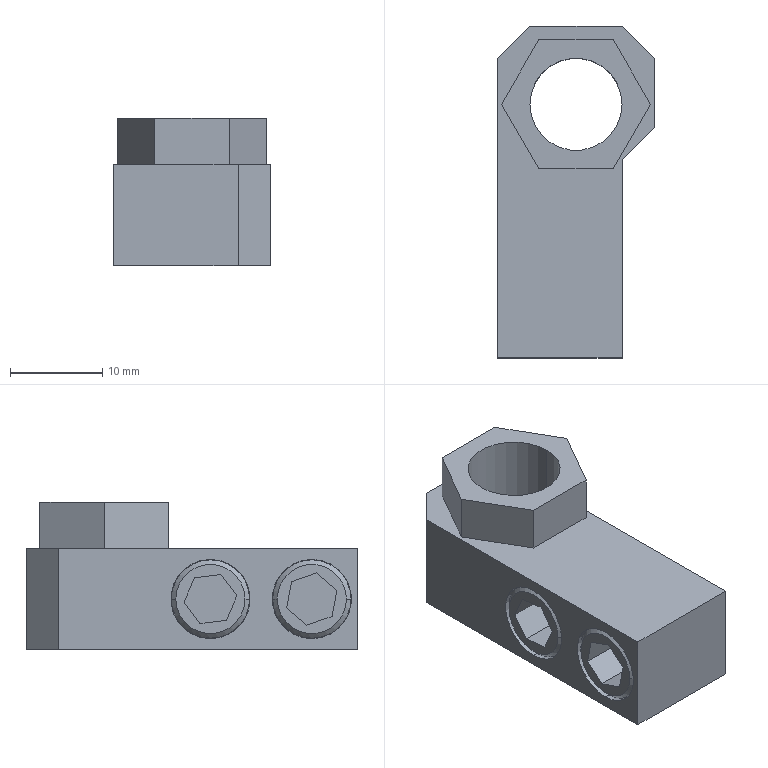Part | NX | 1 solid | 49 faces | box 17 x 36 x 16 mm | volume 4849 mm3 | plane 35 | cylinder 10 | cone 4 | commonest cylinder face diameters 8.5 x4 8.6 x4 10 x2
STEP:
#1=CARTESIAN_POINT('',(0.,27.5,10.5));
#2=VERTEX_POINT('',#1);
#3=CARTESIAN_POINT('',(-10.,27.5,10.5));
#4=VERTEX_POINT('',#3);
#5=CARTESIAN_POINT('',(-5.,27.5,10.5));
#6=DIRECTION('',(0.,0.,1.));
#7=DIRECTION('',(1.,0.,0.));
#8=AXIS2_PLACEMENT_3D('',#5,#6,#7);
#9=CIRCLE('',#8,5.);
#10=EDGE_CURVE('',#2,#4,#9,.T.);
#11=ORIENTED_EDGE('',*,*,#10,.T.);
#12=CARTESIAN_POINT('',(-10.,27.5,-5.5));
#13=VERTEX_POINT('',#12);
#14=CARTESIAN_POINT('',(-10.,27.5,-5.5));
#15=DIRECTION('',(0.,0.,1.));
#16=VECTOR('',#15,1000.);
#17=LINE('',#14,#16);
#18=EDGE_CURVE('',#4,#13,#17,.F.);
#19=ORIENTED_EDGE('',*,*,#18,.T.);
#20=CARTESIAN_POINT('',(0.,27.5,-5.5));
#21=VERTEX_POINT('',#20);
#22=CARTESIAN_POINT('',(-5.,27.5,-5.5));
#23=DIRECTION('',(0.,0.,1.));
#24=DIRECTION('',(1.,0.,0.));
#25=AXIS2_PLACEMENT_3D('',#22,#23,#24);
#26=CIRCLE('',#25,5.);
#27=EDGE_CURVE('',#21,#13,#26,.T.);
#28=ORIENTED_EDGE('',*,*,#27,.F.);
#29=CARTESIAN_POINT('',(0.,27.5,-5.5));
#30=DIRECTION('',(0.,0.,1.));
#31=VECTOR('',#30,1000.);
#32=LINE('',#29,#31);
#33=EDGE_CURVE('',#2,#21,#32,.F.);
#34=ORIENTED_EDGE('',*,*,#33,.F.);
#35=EDGE_LOOP('',(#11,#19,#28,#34));
#36=FACE_BOUND('',#35,.T.);
#37=CARTESIAN_POINT('',(-5.,27.5,-5.5));
#38=DIRECTION('',(0.,0.,1.));
#39=DIRECTION('',(1.,0.,0.));
#40=AXIS2_PLACEMENT_3D('',#37,#38,#39);
#41=CYLINDRICAL_SURFACE('',#40,5.);
#42=ADVANCED_FACE('',(#36),#41,.F.);
#43=CARTESIAN_POINT('',(-13.5,8.75,0.));
#44=VERTEX_POINT('',#43);
#45=CARTESIAN_POINT('',(-13.5,1.25,0.));
#46=VERTEX_POINT('',#45);
#47=CARTESIAN_POINT('',(-13.5,5.,0.));
#48=DIRECTION('',(-1.,0.,0.));
#49=DIRECTION('',(0.,0.,1.));
#50=AXIS2_PLACEMENT_3D('',#47,#48,#49);
#51=CIRCLE('',#50,3.75);
#52=EDGE_CURVE('',#44,#46,#51,.T.);
#53=ORIENTED_EDGE('',*,*,#52,.F.);
#54=CARTESIAN_POINT('',(-13.,9.25,0.));
#55=VERTEX_POINT('',#54);
#56=CARTESIAN_POINT('',(-13.5,8.75,0.));
#57=DIRECTION('',(0.7071,0.7071,0.));
#58=VECTOR('',#57,1000.);
#59=LINE('',#56,#58);
#60=EDGE_CURVE('',#44,#55,#59,.T.);
#61=ORIENTED_EDGE('',*,*,#60,.T.);
#62=CARTESIAN_POINT('',(-13.,5.,-4.25));
#63=VERTEX_POINT('',#62);
#64=CARTESIAN_POINT('',(-13.,5.,0.));
#65=DIRECTION('',(1.,0.,0.));
#66=DIRECTION('',(0.,0.,1.));
#67=AXIS2_PLACEMENT_3D('',#64,#65,#66);
#68=CIRCLE('',#67,4.25);
#69=EDGE_CURVE('',#63,#55,#68,.T.);
#70=ORIENTED_EDGE('',*,*,#69,.F.);
#71=CARTESIAN_POINT('',(-13.,0.75,0.));
#72=VERTEX_POINT('',#71);
#73=CARTESIAN_POINT('',(-13.,5.,0.));
#74=DIRECTION('',(1.,0.,0.));
#75=DIRECTION('',(0.,0.,1.));
#76=AXIS2_PLACEMENT_3D('',#73,#74,#75);
#77=CIRCLE('',#76,4.25);
#78=EDGE_CURVE('',#72,#63,#77,.T.);
#79=ORIENTED_EDGE('',*,*,#78,.F.);
#80=CARTESIAN_POINT('',(-13.5,1.25,0.));
#81=DIRECTION('',(0.7071,-0.7071,0.));
#82=VECTOR('',#81,1000.);
#83=LINE('',#80,#82);
#84=EDGE_CURVE('',#46,#72,#83,.T.);
#85=ORIENTED_EDGE('',*,*,#84,.F.);
#86=EDGE_LOOP('',(#53,#61,#70,#79,#85));
#87=FACE_BOUND('',#86,.T.);
#88=CARTESIAN_POINT('',(-13.5,5.,0.));
#89=DIRECTION('',(1.,0.,0.));
#90=DIRECTION('',(0.,-1.,0.));
#91=AXIS2_PLACEMENT_3D('',#88,#89,#90);
#92=CONICAL_SURFACE('',#91,3.75,0.7854);
#93=ADVANCED_FACE('',(#87),#92,.T.);
#94=CARTESIAN_POINT('',(-13.5,19.75,0.));
#95=VERTEX_POINT('',#94);
#96=CARTESIAN_POINT('',(-13.5,12.25,0.));
#97=VERTEX_POINT('',#96);
#98=CARTESIAN_POINT('',(-13.5,16.,0.));
#99=DIRECTION('',(-1.,0.,0.));
#100=DIRECTION('',(0.,0.,1.));
#101=AXIS2_PLACEMENT_3D('',#98,#99,#100);
#102=CIRCLE('',#101,3.75);
#103=EDGE_CURVE('',#95,#97,#102,.T.);
#104=ORIENTED_EDGE('',*,*,#103,.F.);
#105=CARTESIAN_POINT('',(-13.,20.25,0.));
#106=VERTEX_POINT('',#105);
#107=CARTESIAN_POINT('',(-13.5,19.75,0.));
#108=DIRECTION('',(0.7071,0.7071,0.));
#109=VECTOR('',#108,1000.);
#110=LINE('',#107,#109);
#111=EDGE_CURVE('',#95,#106,#110,.T.);
#112=ORIENTED_EDGE('',*,*,#111,.T.);
#113=CARTESIAN_POINT('',(-13.,16.,-4.25));
#114=VERTEX_POINT('',#113);
#115=CARTESIAN_POINT('',(-13.,16.,0.));
#116=DIRECTION('',(1.,0.,0.));
#117=DIRECTION('',(0.,0.,1.));
#118=AXIS2_PLACEMENT_3D('',#115,#116,#117);
#119=CIRCLE('',#118,4.25);
#120=EDGE_CURVE('',#114,#106,#119,.T.);
#121=ORIENTED_EDGE('',*,*,#120,.F.);
#122=CARTESIAN_POINT('',(-13.,11.75,0.));
#123=VERTEX_POINT('',#122);
#124=CARTESIAN_POINT('',(-13.,16.,0.));
#125=DIRECTION('',(1.,0.,0.));
#126=DIRECTION('',(0.,0.,1.));
#127=AXIS2_PLACEMENT_3D('',#124,#125,#126);
#128=CIRCLE('',#127,4.25);
#129=EDGE_CURVE('',#123,#114,#128,.T.);
#130=ORIENTED_EDGE('',*,*,#129,.F.);
#131=CARTESIAN_POINT('',(-13.5,12.25,0.));
#132=DIRECTION('',(0.7071,-0.7071,0.));
#133=VECTOR('',#132,1000.);
#134=LINE('',#131,#133);
#135=EDGE_CURVE('',#97,#123,#134,.T.);
#136=ORIENTED_EDGE('',*,*,#135,.F.);
#137=EDGE_LOOP('',(#104,#112,#121,#130,#136));
#138=FACE_BOUND('',#137,.T.);
#139=CARTESIAN_POINT('',(-13.5,16.,0.));
#140=DIRECTION('',(1.,0.,0.));
#141=DIRECTION('',(0.,-1.,0.));
#142=AXIS2_PLACEMENT_3D('',#139,#140,#141);
#143=CONICAL_SURFACE('',#142,3.75,0.7854);
#144=ADVANCED_FACE('',(#138),#143,.T.);
#145=CARTESIAN_POINT('',(-13.,16.,4.25));
#146=VERTEX_POINT('',#145);
#147=CARTESIAN_POINT('',(-13.,16.,0.));
#148=DIRECTION('',(1.,0.,0.));
#149=DIRECTION('',(0.,0.,1.));
#150=AXIS2_PLACEMENT_3D('',#147,#148,#149);
#151=CIRCLE('',#150,4.25);
#152=EDGE_CURVE('',#106,#146,#151,.T.);
#153=ORIENTED_EDGE('',*,*,#152,.T.);
#154=CARTESIAN_POINT('',(-11.5,16.,4.25));
#155=VERTEX_POINT('',#154);
#156=CARTESIAN_POINT('',(-13.5,16.,4.25));
#157=DIRECTION('',(1.,0.,0.));
#158=VECTOR('',#157,1000.);
#159=LINE('',#156,#158);
#160=EDGE_CURVE('',#146,#155,#159,.T.);
#161=ORIENTED_EDGE('',*,*,#160,.T.);
#162=CARTESIAN_POINT('',(-11.5,16.,-4.25));
#163=VERTEX_POINT('',#162);
#164=CARTESIAN_POINT('',(-11.5,16.,0.));
#165=DIRECTION('',(-1.,0.,0.));
#166=DIRECTION('',(0.,0.,1.));
#167=AXIS2_PLACEMENT_3D('',#164,#165,#166);
#168=CIRCLE('',#167,4.25);
#169=EDGE_CURVE('',#155,#163,#168,.T.);
#170=ORIENTED_EDGE('',*,*,#169,.T.);
#171=CARTESIAN_POINT('',(-13.5,16.,-4.25));
#172=DIRECTION('',(1.,0.,0.));
#173=VECTOR('',#172,1000.);
#174=LINE('',#171,#173);
#175=EDGE_CURVE('',#114,#163,#174,.T.);
#176=ORIENTED_EDGE('',*,*,#175,.F.);
#177=ORIENTED_EDGE('',*,*,#120,.T.);
#178=EDGE_LOOP('',(#153,#161,#170,#176,#177));
#179=FACE_BOUND('',#178,.T.);
#180=CARTESIAN_POINT('',(-13.5,16.,0.));
#181=DIRECTION('',(1.,0.,0.));
#182=DIRECTION('',(0.,0.,-1.));
#183=AXIS2_PLACEMENT_3D('',#180,#181,#182);
#184=CYLINDRICAL_SURFACE('',#183,4.25);
#185=ADVANCED_FACE('',(#179),#184,.T.);
#186=CARTESIAN_POINT('',(-13.,5.,4.25));
#187=VERTEX_POINT('',#186);
#188=CARTESIAN_POINT('',(-13.,5.,0.));
#189=DIRECTION('',(1.,0.,0.));
#190=DIRECTION('',(0.,0.,1.));
#191=AXIS2_PLACEMENT_3D('',#188,#189,#190);
#192=CIRCLE('',#191,4.25);
#193=EDGE_CURVE('',#55,#187,#192,.T.);
#194=ORIENTED_EDGE('',*,*,#193,.T.);
#195=CARTESIAN_POINT('',(-11.5,5.,4.25));
#196=VERTEX_POINT('',#195);
#197=CARTESIAN_POINT('',(-13.5,5.,4.25));
#198=DIRECTION('',(1.,0.,0.));
#199=VECTOR('',#198,1000.);
#200=LINE('',#197,#199);
#201=EDGE_CURVE('',#187,#196,#200,.T.);
#202=ORIENTED_EDGE('',*,*,#201,.T.);
#203=CARTESIAN_POINT('',(-11.5,5.,-4.25));
#204=VERTEX_POINT('',#203);
#205=CARTESIAN_POINT('',(-11.5,5.,0.));
#206=DIRECTION('',(-1.,0.,0.));
#207=DIRECTION('',(0.,0.,1.));
#208=AXIS2_PLACEMENT_3D('',#205,#206,#207);
#209=CIRCLE('',#208,4.25);
#210=EDGE_CURVE('',#196,#204,#209,.T.);
#211=ORIENTED_EDGE('',*,*,#210,.T.);
#212=CARTESIAN_POINT('',(-13.5,5.,-4.25));
#213=DIRECTION('',(1.,0.,0.));
#214=VECTOR('',#213,1000.);
#215=LINE('',#212,#214);
#216=EDGE_CURVE('',#63,#204,#215,.T.);
#217=ORIENTED_EDGE('',*,*,#216,.F.);
#218=ORIENTED_EDGE('',*,*,#69,.T.);
#219=EDGE_LOOP('',(#194,#202,#211,#217,#218));
#220=FACE_BOUND('',#219,.T.);
#221=CARTESIAN_POINT('',(-13.5,5.,0.));
#222=DIRECTION('',(1.,0.,0.));
#223=DIRECTION('',(0.,0.,-1.));
#224=AXIS2_PLACEMENT_3D('',#221,#222,#223);
#225=CYLINDRICAL_SURFACE('',#224,4.25);
#226=ADVANCED_FACE('',(#220),#225,.T.);
#227=CARTESIAN_POINT('',(-13.5,16.,4.3));
#228=VERTEX_POINT('',#227);
#229=CARTESIAN_POINT('',(-13.5,16.,-4.3));
#230=VERTEX_POINT('',#229);
#231=CARTESIAN_POINT('',(-13.5,16.,0.));
#232=DIRECTION('',(-1.,0.,0.));
#233=DIRECTION('',(0.,0.,1.));
#234=AXIS2_PLACEMENT_3D('',#231,#232,#233);
#235=CIRCLE('',#234,4.3);
#236=EDGE_CURVE('',#228,#230,#235,.T.);
#237=ORIENTED_EDGE('',*,*,#236,.T.);
#238=CARTESIAN_POINT('',(-11.5,16.,-4.3));
#239=VERTEX_POINT('',#238);
#240=CARTESIAN_POINT('',(-11.5,16.,-4.3));
#241=DIRECTION('',(-1.,0.,0.));
#242=VECTOR('',#241,1000.);
#243=LINE('',#240,#242);
#244=EDGE_CURVE('',#239,#230,#243,.T.);
#245=ORIENTED_EDGE('',*,*,#244,.F.);
#246=CARTESIAN_POINT('',(-11.5,16.,4.3));
#247=VERTEX_POINT('',#246);
#248=CARTESIAN_POINT('',(-11.5,16.,0.));
#249=DIRECTION('',(-1.,0.,0.));
#250=DIRECTION('',(0.,0.,1.));
#251=AXIS2_PLACEMENT_3D('',#248,#249,#250);
#252=CIRCLE('',#251,4.3);
#253=EDGE_CURVE('',#247,#239,#252,.T.);
#254=ORIENTED_EDGE('',*,*,#253,.F.);
#255=CARTESIAN_POINT('',(-11.5,16.,4.3));
#256=DIRECTION('',(-1.,0.,0.));
#257=VECTOR('',#256,1000.);
#258=LINE('',#255,#257);
#259=EDGE_CURVE('',#247,#228,#258,.T.);
#260=ORIENTED_EDGE('',*,*,#259,.T.);
#261=EDGE_LOOP('',(#237,#245,#254,#260));
#262=FACE_BOUND('',#261,.T.);
#263=CARTESIAN_POINT('',(-11.5,16.,0.));
#264=DIRECTION('',(-1.,0.,0.));
#265=DIRECTION('',(0.,0.,1.));
#266=AXIS2_PLACEMENT_3D('',#263,#264,#265);
#267=CYLINDRICAL_SURFACE('',#266,4.3);
#268=ADVANCED_FACE('',(#262),#267,.F.);
#269=CARTESIAN_POINT('',(-13.5,5.,4.3));
#270=VERTEX_POINT('',#269);
#271=CARTESIAN_POINT('',(-13.5,5.,-4.3));
#272=VERTEX_POINT('',#271);
#273=CARTESIAN_POINT('',(-13.5,5.,0.));
#274=DIRECTION('',(-1.,0.,0.));
#275=DIRECTION('',(0.,0.,1.));
#276=AXIS2_PLACEMENT_3D('',#273,#274,#275);
#277=CIRCLE('',#276,4.3);
#278=EDGE_CURVE('',#270,#272,#277,.T.);
#279=ORIENTED_EDGE('',*,*,#278,.T.);
#280=CARTESIAN_POINT('',(-11.5,5.,-4.3));
#281=VERTEX_POINT('',#280);
#282=CARTESIAN_POINT('',(-11.5,5.,-4.3));
#283=DIRECTION('',(-1.,0.,0.));
#284=VECTOR('',#283,1000.);
#285=LINE('',#282,#284);
#286=EDGE_CURVE('',#272,#281,#285,.F.);
#287=ORIENTED_EDGE('',*,*,#286,.T.);
#288=CARTESIAN_POINT('',(-11.5,5.,4.3));
#289=VERTEX_POINT('',#288);
#290=CARTESIAN_POINT('',(-11.5,5.,0.));
#291=DIRECTION('',(-1.,0.,0.));
#292=DIRECTION('',(0.,0.,1.));
#293=AXIS2_PLACEMENT_3D('',#290,#291,#292);
#294=CIRCLE('',#293,4.3);
#295=EDGE_CURVE('',#289,#281,#294,.T.);
#296=ORIENTED_EDGE('',*,*,#295,.F.);
#297=CARTESIAN_POINT('',(-11.5,5.,4.3));
#298=DIRECTION('',(-1.,0.,0.));
#299=VECTOR('',#298,1000.);
#300=LINE('',#297,#299);
#301=EDGE_CURVE('',#270,#289,#300,.F.);
#302=ORIENTED_EDGE('',*,*,#301,.F.);
#303=EDGE_LOOP('',(#279,#287,#296,#302));
#304=FACE_BOUND('',#303,.T.);
#305=CARTESIAN_POINT('',(-11.5,5.,0.));
#306=DIRECTION('',(-1.,0.,0.));
#307=DIRECTION('',(0.,0.,1.));
#308=AXIS2_PLACEMENT_3D('',#305,#306,#307);
#309=CYLINDRICAL_SURFACE('',#308,4.3);
#310=ADVANCED_FACE('',(#304),#309,.F.);
#311=CARTESIAN_POINT('',(0.,0.,5.5));
#312=VERTEX_POINT('',#311);
#313=CARTESIAN_POINT('',(0.,21.5,5.5));
#314=VERTEX_POINT('',#313);
#315=CARTESIAN_POINT('',(0.,0.,5.5));
#316=DIRECTION('',(0.,1.,0.));
#317=VECTOR('',#316,1000.);
#318=LINE('',#315,#317);
#319=EDGE_CURVE('',#312,#314,#318,.T.);
#320=ORIENTED_EDGE('',*,*,#319,.T.);
#321=CARTESIAN_POINT('',(3.5,25.,5.5));
#322=VERTEX_POINT('',#321);
#323=CARTESIAN_POINT('',(3.5,25.,5.5));
#324=DIRECTION('',(0.7071,0.7071,0.));
#325=VECTOR('',#324,1000.);
#326=LINE('',#323,#325);
#327=EDGE_CURVE('',#314,#322,#326,.T.);
#328=ORIENTED_EDGE('',*,*,#327,.T.);
#329=CARTESIAN_POINT('',(3.5,32.5,5.5));
#330=VERTEX_POINT('',#329);
#331=CARTESIAN_POINT('',(3.5,36.,5.5));
#332=DIRECTION('',(0.,1.,0.));
#333=VECTOR('',#332,1000.);
#334=LINE('',#331,#333);
#335=EDGE_CURVE('',#322,#330,#334,.T.);
#336=ORIENTED_EDGE('',*,*,#335,.T.);
#337=CARTESIAN_POINT('',(0.,36.,5.5));
#338=VERTEX_POINT('',#337);
#339=CARTESIAN_POINT('',(0.,36.,5.5));
#340=DIRECTION('',(-0.7071,0.7071,0.));
#341=VECTOR('',#340,1000.);
#342=LINE('',#339,#341);
#343=EDGE_CURVE('',#330,#338,#342,.T.);
#344=ORIENTED_EDGE('',*,*,#343,.T.);
#345=CARTESIAN_POINT('',(-10.,36.,5.5));
#346=VERTEX_POINT('',#345);
#347=CARTESIAN_POINT('',(3.5,36.,5.5));
#348=DIRECTION('',(-1.,0.,0.));
#349=VECTOR('',#348,1000.);
#350=LINE('',#347,#349);
#351=EDGE_CURVE('',#338,#346,#350,.T.);
#352=ORIENTED_EDGE('',*,*,#351,.T.);
#353=CARTESIAN_POINT('',(-13.5,32.5,5.5));
#354=VERTEX_POINT('',#353);
#355=CARTESIAN_POINT('',(-13.5,32.5,5.5));
#356=DIRECTION('',(-0.7071,-0.7071,0.));
#357=VECTOR('',#356,1000.);
#358=LINE('',#355,#357);
#359=EDGE_CURVE('',#346,#354,#358,.T.);
#360=ORIENTED_EDGE('',*,*,#359,.T.);
#361=CARTESIAN_POINT('',(-13.5,0.,5.5));
#362=VERTEX_POINT('',#361);
#363=CARTESIAN_POINT('',(-13.5,0.,5.5));
#364=DIRECTION('',(0.,-1.,0.));
#365=VECTOR('',#364,1000.);
#366=LINE('',#363,#365);
#367=EDGE_CURVE('',#354,#362,#366,.T.);
#368=ORIENTED_EDGE('',*,*,#367,.T.);
#369=CARTESIAN_POINT('',(0.,0.,5.5));
#370=DIRECTION('',(1.,0.,0.));
#371=VECTOR('',#370,1000.);
#372=LINE('',#369,#371);
#373=EDGE_CURVE('',#362,#312,#372,.T.);
#374=ORIENTED_EDGE('',*,*,#373,.T.);
#375=EDGE_LOOP('',(#320,#328,#336,#344,#352,#360,#368,#374));
#376=FACE_BOUND('',#375,.T.);
#377=CARTESIAN_POINT('',(-13.083,27.5,5.5));
#378=VERTEX_POINT('',#377);
#379=CARTESIAN_POINT('',(-9.041,20.5,5.5));
#380=VERTEX_POINT('',#379);
#381=CARTESIAN_POINT('',(-13.083,27.5,5.5));
#382=DIRECTION('',(0.5,-0.866,0.));
#383=VECTOR('',#382,1000.);
#384=LINE('',#381,#383);
#385=EDGE_CURVE('',#378,#380,#384,.T.);
#386=ORIENTED_EDGE('',*,*,#385,.F.);
#387=CARTESIAN_POINT('',(-9.041,34.5,5.5));
#388=VERTEX_POINT('',#387);
#389=CARTESIAN_POINT('',(-9.041,34.5,5.5));
#390=DIRECTION('',(-0.5,-0.866,0.));
#391=VECTOR('',#390,1000.);
#392=LINE('',#389,#391);
#393=EDGE_CURVE('',#388,#378,#392,.T.);
#394=ORIENTED_EDGE('',*,*,#393,.F.);
#395=CARTESIAN_POINT('',(-0.9585,34.5,5.5));
#396=VERTEX_POINT('',#395);
#397=CARTESIAN_POINT('',(-0.9585,34.5,5.5));
#398=DIRECTION('',(-1.,0.,0.));
#399=VECTOR('',#398,1000.);
#400=LINE('',#397,#399);
#401=EDGE_CURVE('',#396,#388,#400,.T.);
#402=ORIENTED_EDGE('',*,*,#401,.F.);
#403=CARTESIAN_POINT('',(3.083,27.5,5.5));
#404=VERTEX_POINT('',#403);
#405=CARTESIAN_POINT('',(3.083,27.5,5.5));
#406=DIRECTION('',(-0.5,0.866,0.));
#407=VECTOR('',#406,1000.);
#408=LINE('',#405,#407);
#409=EDGE_CURVE('',#404,#396,#408,.T.);
#410=ORIENTED_EDGE('',*,*,#409,.F.);
#411=CARTESIAN_POINT('',(-0.9585,20.5,5.5));
#412=VERTEX_POINT('',#411);
#413=CARTESIAN_POINT('',(-0.9585,20.5,5.5));
#414=DIRECTION('',(0.5,0.866,0.));
#415=VECTOR('',#414,1000.);
#416=LINE('',#413,#415);
#417=EDGE_CURVE('',#412,#404,#416,.T.);
#418=ORIENTED_EDGE('',*,*,#417,.F.);
#419=CARTESIAN_POINT('',(-9.041,20.5,5.5));
#420=DIRECTION('',(1.,0.,0.));
#421=VECTOR('',#420,1000.);
#422=LINE('',#419,#421);
#423=EDGE_CURVE('',#380,#412,#422,.T.);
#424=ORIENTED_EDGE('',*,*,#423,.F.);
#425=EDGE_LOOP('',(#386,#394,#402,#410,#418,#424));
#426=FACE_BOUND('',#425,.T.);
#427=CARTESIAN_POINT('',(0.,21.5,5.5));
#428=DIRECTION('',(0.,0.,-1.));
#429=DIRECTION('',(0.,-1.,0.));
#430=AXIS2_PLACEMENT_3D('',#427,#428,#429);
#431=PLANE('',#430);
#432=ADVANCED_FACE('',(#376,#426),#431,.F.);
#433=ORIENTED_EDGE('',*,*,#253,.T.);
#434=CARTESIAN_POINT('',(-11.5,16.,0.));
#435=DIRECTION('',(-1.,0.,0.));
#436=DIRECTION('',(0.,0.,1.));
#437=AXIS2_PLACEMENT_3D('',#434,#435,#436);
#438=CIRCLE('',#437,4.3);
#439=EDGE_CURVE('',#239,#247,#438,.T.);
#440=ORIENTED_EDGE('',*,*,#439,.T.);
#441=EDGE_LOOP('',(#433,#440));
#442=FACE_BOUND('',#441,.T.);
#443=ORIENTED_EDGE('',*,*,#169,.F.);
#444=CARTESIAN_POINT('',(-11.5,16.,0.));
#445=DIRECTION('',(-1.,0.,0.));
#446=DIRECTION('',(0.,0.,1.));
#447=AXIS2_PLACEMENT_3D('',#444,#445,#446);
#448=CIRCLE('',#447,4.25);
#449=EDGE_CURVE('',#163,#155,#448,.T.);
#450=ORIENTED_EDGE('',*,*,#449,.F.);
#451=EDGE_LOOP('',(#443,#450));
#452=FACE_BOUND('',#451,.T.);
#453=CARTESIAN_POINT('',(-11.5,16.,0.));
#454=DIRECTION('',(-1.,0.,0.));
#455=DIRECTION('',(0.,0.,1.));
#456=AXIS2_PLACEMENT_3D('',#453,#454,#455);
#457=PLANE('',#456);
#458=ADVANCED_FACE('',(#442,#452),#457,.T.);
#459=CARTESIAN_POINT('',(-11.5,5.,0.));
#460=DIRECTION('',(-1.,0.,0.));
#461=DIRECTION('',(0.,0.,1.));
#462=AXIS2_PLACEMENT_3D('',#459,#460,#461);
#463=CIRCLE('',#462,4.3);
#464=EDGE_CURVE('',#281,#289,#463,.T.);
#465=ORIENTED_EDGE('',*,*,#464,.T.);
#466=ORIENTED_EDGE('',*,*,#295,.T.);
#467=EDGE_LOOP('',(#465,#466));
#468=FACE_BOUND('',#467,.T.);
#469=CARTESIAN_POINT('',(-11.5,5.,0.));
#470=DIRECTION('',(-1.,0.,0.));
#471=DIRECTION('',(0.,0.,1.));
#472=AXIS2_PLACEMENT_3D('',#469,#470,#471);
#473=CIRCLE('',#472,4.25);
#474=EDGE_CURVE('',#204,#196,#473,.T.);
#475=ORIENTED_EDGE('',*,*,#474,.F.);
#476=ORIENTED_EDGE('',*,*,#210,.F.);
#477=EDGE_LOOP('',(#475,#476));
#478=FACE_BOUND('',#477,.T.);
#479=CARTESIAN_POINT('',(-11.5,5.,0.));
#480=DIRECTION('',(-1.,0.,0.));
#481=DIRECTION('',(0.,0.,1.));
#482=AXIS2_PLACEMENT_3D('',#479,#480,#481);
#483=PLANE('',#482);
#484=ADVANCED_FACE('',(#468,#478),#483,.T.);
#485=CARTESIAN_POINT('',(0.,0.,-5.5));
#486=VERTEX_POINT('',#485);
#487=CARTESIAN_POINT('',(0.,21.5,-5.5));
#488=VERTEX_POINT('',#487);
#489=CARTESIAN_POINT('',(0.,0.,-5.5));
#490=DIRECTION('',(0.,1.,0.));
#491=VECTOR('',#490,1000.);
#492=LINE('',#489,#491);
#493=EDGE_CURVE('',#486,#488,#492,.T.);
#494=ORIENTED_EDGE('',*,*,#493,.T.);
#495=CARTESIAN_POINT('',(0.,21.5,5.5));
#496=DIRECTION('',(0.,0.,-1.));
#497=VECTOR('',#496,1000.);
#498=LINE('',#495,#497);
#499=EDGE_CURVE('',#314,#488,#498,.T.);
#500=ORIENTED_EDGE('',*,*,#499,.F.);
#501=ORIENTED_EDGE('',*,*,#319,.F.);
#502=CARTESIAN_POINT('',(0.,0.,5.5));
#503=DIRECTION('',(0.,0.,-1.));
#504=VECTOR('',#503,1000.);
#505=LINE('',#502,#504);
#506=EDGE_CURVE('',#312,#486,#505,.T.);
#507=ORIENTED_EDGE('',*,*,#506,.T.);
#508=EDGE_LOOP('',(#494,#500,#501,#507));
#509=FACE_BOUND('',#508,.T.);
#510=CARTESIAN_POINT('',(0.,0.,5.5));
#511=DIRECTION('',(-1.,0.,0.));
#512=DIRECTION('',(0.,0.,1.));
#513=AXIS2_PLACEMENT_3D('',#510,#511,#512);
#514=PLANE('',#513);
#515=ADVANCED_FACE('',(#509),#514,.F.);
#516=ORIENTED_EDGE('',*,*,#335,.F.);
#517=CARTESIAN_POINT('',(3.5,25.,-5.5));
#518=VERTEX_POINT('',#517);
#519=CARTESIAN_POINT('',(3.5,25.,5.5));
#520=DIRECTION('',(0.,0.,-1.));
#521=VECTOR('',#520,1000.);
#522=LINE('',#519,#521);
#523=EDGE_CURVE('',#322,#518,#522,.T.);
#524=ORIENTED_EDGE('',*,*,#523,.T.);
#525=CARTESIAN_POINT('',(3.5,32.5,-5.5));
#526=VERTEX_POINT('',#525);
#527=CARTESIAN_POINT('',(3.5,36.,-5.5));
#528=DIRECTION('',(0.,1.,0.));
#529=VECTOR('',#528,1000.);
#530=LINE('',#527,#529);
#531=EDGE_CURVE('',#518,#526,#530,.T.);
#532=ORIENTED_EDGE('',*,*,#531,.T.);
#533=CARTESIAN_POINT('',(3.5,32.5,5.5));
#534=DIRECTION('',(0.,0.,1.));
#535=VECTOR('',#534,1000.);
#536=LINE('',#533,#535);
#537=EDGE_CURVE('',#526,#330,#536,.T.);
#538=ORIENTED_EDGE('',*,*,#537,.T.);
#539=EDGE_LOOP('',(#516,#524,#532,#538));
#540=FACE_BOUND('',#539,.T.);
#541=CARTESIAN_POINT('',(3.5,36.,5.5));
#542=DIRECTION('',(-1.,0.,0.));
#543=DIRECTION('',(0.,1.,0.));
#544=AXIS2_PLACEMENT_3D('',#541,#542,#543);
#545=PLANE('',#544);
#546=ADVANCED_FACE('',(#540),#545,.F.);
#547=CARTESIAN_POINT('',(0.,36.,-5.5));
#548=VERTEX_POINT('',#547);
#549=CARTESIAN_POINT('',(-10.,36.,-5.5));
#550=VERTEX_POINT('',#549);
#551=CARTESIAN_POINT('',(3.5,36.,-5.5));
#552=DIRECTION('',(-1.,0.,0.));
#553=VECTOR('',#552,1000.);
#554=LINE('',#551,#553);
#555=EDGE_CURVE('',#548,#550,#554,.T.);
#556=ORIENTED_EDGE('',*,*,#555,.T.);
#557=CARTESIAN_POINT('',(-10.,36.,5.5));
#558=DIRECTION('',(0.,0.,1.));
#559=VECTOR('',#558,1000.);
#560=LINE('',#557,#559);
#561=EDGE_CURVE('',#550,#346,#560,.T.);
#562=ORIENTED_EDGE('',*,*,#561,.T.);
#563=ORIENTED_EDGE('',*,*,#351,.F.);
#564=CARTESIAN_POINT('',(0.,36.,5.5));
#565=DIRECTION('',(0.,0.,-1.));
#566=VECTOR('',#565,1000.);
#567=LINE('',#564,#566);
#568=EDGE_CURVE('',#338,#548,#567,.T.);
#569=ORIENTED_EDGE('',*,*,#568,.T.);
#570=EDGE_LOOP('',(#556,#562,#563,#569));
#571=FACE_BOUND('',#570,.T.);
#572=CARTESIAN_POINT('',(3.5,36.,5.5));
#573=DIRECTION('',(0.,-1.,0.));
#574=DIRECTION('',(0.,0.,-1.));
#575=AXIS2_PLACEMENT_3D('',#572,#573,#574);
#576=PLANE('',#575);
#577=ADVANCED_FACE('',(#571),#576,.F.);
#578=ORIENTED_EDGE('',*,*,#367,.F.);
#579=CARTESIAN_POINT('',(-13.5,32.5,-5.5));
#580=VERTEX_POINT('',#579);
#581=CARTESIAN_POINT('',(-13.5,32.5,5.5));
#582=DIRECTION('',(0.,0.,-1.));
#583=VECTOR('',#582,1000.);
#584=LINE('',#581,#583);
#585=EDGE_CURVE('',#354,#580,#584,.T.);
#586=ORIENTED_EDGE('',*,*,#585,.T.);
#587=CARTESIAN_POINT('',(-13.5,0.,-5.5));
#588=VERTEX_POINT('',#587);
#589=CARTESIAN_POINT('',(-13.5,0.,-5.5));
#590=DIRECTION('',(0.,-1.,0.));
#591=VECTOR('',#590,1000.);
#592=LINE('',#589,#591);
#593=EDGE_CURVE('',#580,#588,#592,.T.);
#594=ORIENTED_EDGE('',*,*,#593,.T.);
#595=CARTESIAN_POINT('',(-13.5,0.,5.5));
#596=DIRECTION('',(0.,0.,-1.));
#597=VECTOR('',#596,1000.);
#598=LINE('',#595,#597);
#599=EDGE_CURVE('',#362,#588,#598,.T.);
#600=ORIENTED_EDGE('',*,*,#599,.F.);
#601=EDGE_LOOP('',(#578,#586,#594,#600));
#602=FACE_BOUND('',#601,.T.);
#603=ORIENTED_EDGE('',*,*,#236,.F.);
#604=CARTESIAN_POINT('',(-13.5,16.,0.));
#605=DIRECTION('',(-1.,0.,0.));
#606=DIRECTION('',(0.,0.,1.));
#607=AXIS2_PLACEMENT_3D('',#604,#605,#606);
#608=CIRCLE('',#607,4.3);
#609=EDGE_CURVE('',#230,#228,#608,.T.);
#610=ORIENTED_EDGE('',*,*,#609,.F.);
#611=EDGE_LOOP('',(#603,#610));
#612=FACE_BOUND('',#611,.T.);
#613=ORIENTED_EDGE('',*,*,#278,.F.);
#614=CARTESIAN_POINT('',(-13.5,5.,0.));
#615=DIRECTION('',(-1.,0.,0.));
#616=DIRECTION('',(0.,0.,1.));
#617=AXIS2_PLACEMENT_3D('',#614,#615,#616);
#618=CIRCLE('',#617,4.3);
#619=EDGE_CURVE('',#272,#270,#618,.T.);
#620=ORIENTED_EDGE('',*,*,#619,.F.);
#621=EDGE_LOOP('',(#613,#620));
#622=FACE_BOUND('',#621,.T.);
#623=CARTESIAN_POINT('',(-13.5,0.,5.5));
#624=DIRECTION('',(1.,0.,0.));
#625=DIRECTION('',(0.,-1.,0.));
#626=AXIS2_PLACEMENT_3D('',#623,#624,#625);
#627=PLANE('',#626);
#628=ADVANCED_FACE('',(#602,#612,#622),#627,.F.);
#629=CARTESIAN_POINT('',(0.,0.,-5.5));
#630=DIRECTION('',(1.,0.,0.));
#631=VECTOR('',#630,1000.);
#632=LINE('',#629,#631);
#633=EDGE_CURVE('',#588,#486,#632,.T.);
#634=ORIENTED_EDGE('',*,*,#633,.T.);
#635=ORIENTED_EDGE('',*,*,#506,.F.);
#636=ORIENTED_EDGE('',*,*,#373,.F.);
#637=ORIENTED_EDGE('',*,*,#599,.T.);
#638=EDGE_LOOP('',(#634,#635,#636,#637));
#639=FACE_BOUND('',#638,.T.);
#640=CARTESIAN_POINT('',(0.,0.,5.5));
#641=DIRECTION('',(0.,1.,0.));
#642=DIRECTION('',(1.,0.,0.));
#643=AXIS2_PLACEMENT_3D('',#640,#641,#642);
#644=PLANE('',#643);
#645=ADVANCED_FACE('',(#639),#644,.F.);
#646=ORIENTED_EDGE('',*,*,#531,.F.);
#647=CARTESIAN_POINT('',(0.,21.5,-5.5));
#648=DIRECTION('',(-0.7071,-0.7071,0.));
#649=VECTOR('',#648,1000.);
#650=LINE('',#647,#649);
#651=EDGE_CURVE('',#518,#488,#650,.T.);
#652=ORIENTED_EDGE('',*,*,#651,.T.);
#653=ORIENTED_EDGE('',*,*,#493,.F.);
#654=ORIENTED_EDGE('',*,*,#633,.F.);
#655=ORIENTED_EDGE('',*,*,#593,.F.);
#656=CARTESIAN_POINT('',(-12.25,33.75,-5.5));
#657=DIRECTION('',(0.7071,0.7071,0.));
#658=VECTOR('',#657,1000.);
#659=LINE('',#656,#658);
#660=EDGE_CURVE('',#580,#550,#659,.T.);
#661=ORIENTED_EDGE('',*,*,#660,.T.);
#662=ORIENTED_EDGE('',*,*,#555,.F.);
#663=CARTESIAN_POINT('',(7.25,28.75,-5.5));
#664=DIRECTION('',(0.7071,-0.7071,0.));
#665=VECTOR('',#664,1000.);
#666=LINE('',#663,#665);
#667=EDGE_CURVE('',#548,#526,#666,.T.);
#668=ORIENTED_EDGE('',*,*,#667,.T.);
#669=EDGE_LOOP('',(#646,#652,#653,#654,#655,#661,#662,#668));
#670=FACE_BOUND('',#669,.T.);
#671=CARTESIAN_POINT('',(-5.,27.5,-5.5));
#672=DIRECTION('',(0.,0.,1.));
#673=DIRECTION('',(1.,0.,0.));
#674=AXIS2_PLACEMENT_3D('',#671,#672,#673);
#675=CIRCLE('',#674,5.);
#676=EDGE_CURVE('',#13,#21,#675,.T.);
#677=ORIENTED_EDGE('',*,*,#676,.T.);
#678=ORIENTED_EDGE('',*,*,#27,.T.);
#679=EDGE_LOOP('',(#677,#678));
#680=FACE_BOUND('',#679,.T.);
#681=CARTESIAN_POINT('',(0.,21.5,-5.5));
#682=DIRECTION('',(0.,0.,-1.));
#683=DIRECTION('',(0.,-1.,0.));
#684=AXIS2_PLACEMENT_3D('',#681,#682,#683);
#685=PLANE('',#684);
#686=ADVANCED_FACE('',(#670,#680),#685,.T.);
#687=ORIENTED_EDGE('',*,*,#401,.T.);
#688=CARTESIAN_POINT('',(-9.041,34.5,10.5));
#689=VERTEX_POINT('',#688);
#690=CARTESIAN_POINT('',(-9.041,34.5,10.5));
#691=DIRECTION('',(0.,0.,-1.));
#692=VECTOR('',#691,1000.);
#693=LINE('',#690,#692);
#694=EDGE_CURVE('',#689,#388,#693,.T.);
#695=ORIENTED_EDGE('',*,*,#694,.F.);
#696=CARTESIAN_POINT('',(-0.9585,34.5,10.5));
#697=VERTEX_POINT('',#696);
#698=CARTESIAN_POINT('',(-0.9585,34.5,10.5));
#699=DIRECTION('',(-1.,0.,0.));
#700=VECTOR('',#699,1000.);
#701=LINE('',#698,#700);
#702=EDGE_CURVE('',#697,#689,#701,.T.);
#703=ORIENTED_EDGE('',*,*,#702,.F.);
#704=CARTESIAN_POINT('',(-0.9585,34.5,10.5));
#705=DIRECTION('',(0.,0.,-1.));
#706=VECTOR('',#705,1000.);
#707=LINE('',#704,#706);
#708=EDGE_CURVE('',#697,#396,#707,.T.);
#709=ORIENTED_EDGE('',*,*,#708,.T.);
#710=EDGE_LOOP('',(#687,#695,#703,#709));
#711=FACE_BOUND('',#710,.T.);
#712=CARTESIAN_POINT('',(-0.9585,34.5,10.5));
#713=DIRECTION('',(0.,-1.,0.));
#714=DIRECTION('',(0.,0.,-1.));
#715=AXIS2_PLACEMENT_3D('',#712,#713,#714);
#716=PLANE('',#715);
#717=ADVANCED_FACE('',(#711),#716,.F.);
#718=ORIENTED_EDGE('',*,*,#393,.T.);
#719=CARTESIAN_POINT('',(-13.083,27.5,10.5));
#720=VERTEX_POINT('',#719);
#721=CARTESIAN_POINT('',(-13.083,27.5,10.5));
#722=DIRECTION('',(0.,0.,-1.));
#723=VECTOR('',#722,1000.);
#724=LINE('',#721,#723);
#725=EDGE_CURVE('',#720,#378,#724,.T.);
#726=ORIENTED_EDGE('',*,*,#725,.F.);
#727=CARTESIAN_POINT('',(-9.041,34.5,10.5));
#728=DIRECTION('',(-0.5,-0.866,0.));
#729=VECTOR('',#728,1000.);
#730=LINE('',#727,#729);
#731=EDGE_CURVE('',#689,#720,#730,.T.);
#732=ORIENTED_EDGE('',*,*,#731,.F.);
#733=ORIENTED_EDGE('',*,*,#694,.T.);
#734=EDGE_LOOP('',(#718,#726,#732,#733));
#735=FACE_BOUND('',#734,.T.);
#736=CARTESIAN_POINT('',(-9.041,34.5,10.5));
#737=DIRECTION('',(0.866,-0.5,0.));
#738=DIRECTION('',(0.,0.,-1.));
#739=AXIS2_PLACEMENT_3D('',#736,#737,#738);
#740=PLANE('',#739);
#741=ADVANCED_FACE('',(#735),#740,.F.);
#742=ORIENTED_EDGE('',*,*,#343,.F.);
#743=ORIENTED_EDGE('',*,*,#537,.F.);
#744=ORIENTED_EDGE('',*,*,#667,.F.);
#745=ORIENTED_EDGE('',*,*,#568,.F.);
#746=EDGE_LOOP('',(#742,#743,#744,#745));
#747=FACE_BOUND('',#746,.T.);
#748=CARTESIAN_POINT('',(0.,36.,5.5));
#749=DIRECTION('',(-0.7071,-0.7071,0.));
#750=DIRECTION('',(-0.7071,0.7071,0.));
#751=AXIS2_PLACEMENT_3D('',#748,#749,#750);
#752=PLANE('',#751);
#753=ADVANCED_FACE('',(#747),#752,.F.);
#754=ORIENTED_EDGE('',*,*,#52,.T.);
#755=CARTESIAN_POINT('',(-13.5,5.,0.));
#756=DIRECTION('',(-1.,0.,0.));
#757=DIRECTION('',(0.,0.,1.));
#758=AXIS2_PLACEMENT_3D('',#755,#756,#757);
#759=CIRCLE('',#758,3.75);
#760=EDGE_CURVE('',#46,#44,#759,.T.);
#761=ORIENTED_EDGE('',*,*,#760,.T.);
#762=EDGE_LOOP('',(#754,#761));
#763=FACE_BOUND('',#762,.T.);
#764=CARTESIAN_POINT('',(-13.5,2.81,-1.88));
#765=VERTEX_POINT('',#764);
#766=CARTESIAN_POINT('',(-13.5,2.276,0.9565));
#767=VERTEX_POINT('',#766);
#768=CARTESIAN_POINT('',(-13.5,2.81,-1.88));
#769=DIRECTION('',(0.,-0.1848,0.9828));
#770=VECTOR('',#769,1000.);
#771=LINE('',#768,#770);
#772=EDGE_CURVE('',#765,#767,#771,.T.);
#773=ORIENTED_EDGE('',*,*,#772,.F.);
#774=CARTESIAN_POINT('',(-13.5,5.533,-2.837));
#775=VERTEX_POINT('',#774);
#776=CARTESIAN_POINT('',(-13.5,5.533,-2.837));
#777=DIRECTION('',(0.,-0.9435,0.3314));
#778=VECTOR('',#777,1000.);
#779=LINE('',#776,#778);
#780=EDGE_CURVE('',#775,#765,#779,.T.);
#781=ORIENTED_EDGE('',*,*,#780,.F.);
#782=CARTESIAN_POINT('',(-13.5,7.724,-0.9565));
#783=VERTEX_POINT('',#782);
#784=CARTESIAN_POINT('',(-13.5,7.724,-0.9565));
#785=DIRECTION('',(0.,-0.7587,-0.6514));
#786=VECTOR('',#785,1000.);
#787=LINE('',#784,#786);
#788=EDGE_CURVE('',#783,#775,#787,.T.);
#789=ORIENTED_EDGE('',*,*,#788,.F.);
#790=CARTESIAN_POINT('',(-13.5,7.19,1.88));
#791=VERTEX_POINT('',#790);
#792=CARTESIAN_POINT('',(-13.5,7.19,1.88));
#793=DIRECTION('',(0.,0.1848,-0.9828));
#794=VECTOR('',#793,1000.);
#795=LINE('',#792,#794);
#796=EDGE_CURVE('',#791,#783,#795,.T.);
#797=ORIENTED_EDGE('',*,*,#796,.F.);
#798=CARTESIAN_POINT('',(-13.5,4.467,2.837));
#799=VERTEX_POINT('',#798);
#800=CARTESIAN_POINT('',(-13.5,4.467,2.837));
#801=DIRECTION('',(0.,0.9435,-0.3314));
#802=VECTOR('',#801,1000.);
#803=LINE('',#800,#802);
#804=EDGE_CURVE('',#799,#791,#803,.T.);
#805=ORIENTED_EDGE('',*,*,#804,.F.);
#806=CARTESIAN_POINT('',(-13.5,2.276,0.9565));
#807=DIRECTION('',(0.,0.7587,0.6514));
#808=VECTOR('',#807,1000.);
#809=LINE('',#806,#808);
#810=EDGE_CURVE('',#767,#799,#809,.T.);
#811=ORIENTED_EDGE('',*,*,#810,.F.);
#812=EDGE_LOOP('',(#773,#781,#789,#797,#805,#811));
#813=FACE_BOUND('',#812,.T.);
#814=CARTESIAN_POINT('',(-13.5,5.,0.));
#815=DIRECTION('',(-1.,0.,0.));
#816=DIRECTION('',(0.,0.,1.));
#817=AXIS2_PLACEMENT_3D('',#814,#815,#816);
#818=PLANE('',#817);
#819=ADVANCED_FACE('',(#763,#813),#818,.T.);
#820=ORIENTED_EDGE('',*,*,#359,.F.);
#821=ORIENTED_EDGE('',*,*,#561,.F.);
#822=ORIENTED_EDGE('',*,*,#660,.F.);
#823=ORIENTED_EDGE('',*,*,#585,.F.);
#824=EDGE_LOOP('',(#820,#821,#822,#823));
#825=FACE_BOUND('',#824,.T.);
#826=CARTESIAN_POINT('',(-13.5,32.5,5.5));
#827=DIRECTION('',(0.7071,-0.7071,0.));
#828=DIRECTION('',(0.,0.,-1.));
#829=AXIS2_PLACEMENT_3D('',#826,#827,#828);
#830=PLANE('',#829);
#831=ADVANCED_FACE('',(#825),#830,.F.);
#832=ORIENTED_EDGE('',*,*,#103,.T.);
#833=CARTESIAN_POINT('',(-13.5,16.,0.));
#834=DIRECTION('',(-1.,0.,0.));
#835=DIRECTION('',(0.,0.,1.));
#836=AXIS2_PLACEMENT_3D('',#833,#834,#835);
#837=CIRCLE('',#836,3.75);
#838=EDGE_CURVE('',#97,#95,#837,.T.);
#839=ORIENTED_EDGE('',*,*,#838,.T.);
#840=EDGE_LOOP('',(#832,#839));
#841=FACE_BOUND('',#840,.T.);
#842=CARTESIAN_POINT('',(-13.5,14.272,-2.313));
#843=VERTEX_POINT('',#842);
#844=CARTESIAN_POINT('',(-13.5,13.133,0.3401));
#845=VERTEX_POINT('',#844);
#846=CARTESIAN_POINT('',(-13.5,14.272,-2.313));
#847=DIRECTION('',(0.,-0.3945,0.9189));
#848=VECTOR('',#847,1000.);
#849=LINE('',#846,#848);
#850=EDGE_CURVE('',#843,#845,#849,.T.);
#851=ORIENTED_EDGE('',*,*,#850,.F.);
#852=CARTESIAN_POINT('',(-13.5,17.139,-2.653));
#853=VERTEX_POINT('',#852);
#854=CARTESIAN_POINT('',(-13.5,17.139,-2.653));
#855=DIRECTION('',(0.,-0.993,0.1178));
#856=VECTOR('',#855,1000.);
#857=LINE('',#854,#856);
#858=EDGE_CURVE('',#853,#843,#857,.T.);
#859=ORIENTED_EDGE('',*,*,#858,.F.);
#860=CARTESIAN_POINT('',(-13.5,18.867,-0.3401));
#861=VERTEX_POINT('',#860);
#862=CARTESIAN_POINT('',(-13.5,18.867,-0.3401));
#863=DIRECTION('',(0.,-0.5986,-0.8011));
#864=VECTOR('',#863,1000.);
#865=LINE('',#862,#864);
#866=EDGE_CURVE('',#861,#853,#865,.T.);
#867=ORIENTED_EDGE('',*,*,#866,.F.);
#868=CARTESIAN_POINT('',(-13.5,17.728,2.313));
#869=VERTEX_POINT('',#868);
#870=CARTESIAN_POINT('',(-13.5,17.728,2.313));
#871=DIRECTION('',(0.,0.3945,-0.9189));
#872=VECTOR('',#871,1000.);
#873=LINE('',#870,#872);
#874=EDGE_CURVE('',#869,#861,#873,.T.);
#875=ORIENTED_EDGE('',*,*,#874,.F.);
#876=CARTESIAN_POINT('',(-13.5,14.861,2.653));
#877=VERTEX_POINT('',#876);
#878=CARTESIAN_POINT('',(-13.5,14.861,2.653));
#879=DIRECTION('',(0.,0.993,-0.1178));
#880=VECTOR('',#879,1000.);
#881=LINE('',#878,#880);
#882=EDGE_CURVE('',#877,#869,#881,.T.);
#883=ORIENTED_EDGE('',*,*,#882,.F.);
#884=CARTESIAN_POINT('',(-13.5,13.133,0.3401));
#885=DIRECTION('',(0.,0.5986,0.8011));
#886=VECTOR('',#885,1000.);
#887=LINE('',#884,#886);
#888=EDGE_CURVE('',#845,#877,#887,.T.);
#889=ORIENTED_EDGE('',*,*,#888,.F.);
#890=EDGE_LOOP('',(#851,#859,#867,#875,#883,#889));
#891=FACE_BOUND('',#890,.T.);
#892=CARTESIAN_POINT('',(-13.5,16.,0.));
#893=DIRECTION('',(-1.,0.,0.));
#894=DIRECTION('',(0.,0.,1.));
#895=AXIS2_PLACEMENT_3D('',#892,#893,#894);
#896=PLANE('',#895);
#897=ADVANCED_FACE('',(#841,#891),#896,.T.);
#898=ORIENTED_EDGE('',*,*,#850,.T.);
#899=CARTESIAN_POINT('',(-3.5,13.133,0.3401));
#900=VERTEX_POINT('',#899);
#901=CARTESIAN_POINT('',(-3.5,13.133,0.3401));
#902=DIRECTION('',(-1.,0.,0.));
#903=VECTOR('',#902,1000.);
#904=LINE('',#901,#903);
#905=EDGE_CURVE('',#900,#845,#904,.T.);
#906=ORIENTED_EDGE('',*,*,#905,.F.);
#907=CARTESIAN_POINT('',(-3.5,14.272,-2.313));
#908=VERTEX_POINT('',#907);
#909=CARTESIAN_POINT('',(-3.5,14.272,-2.313));
#910=DIRECTION('',(0.,-0.3945,0.9189));
#911=VECTOR('',#910,1000.);
#912=LINE('',#909,#911);
#913=EDGE_CURVE('',#908,#900,#912,.T.);
#914=ORIENTED_EDGE('',*,*,#913,.F.);
#915=CARTESIAN_POINT('',(-3.5,14.272,-2.313));
#916=DIRECTION('',(-1.,0.,0.));
#917=VECTOR('',#916,1000.);
#918=LINE('',#915,#917);
#919=EDGE_CURVE('',#908,#843,#918,.T.);
#920=ORIENTED_EDGE('',*,*,#919,.T.);
#921=EDGE_LOOP('',(#898,#906,#914,#920));
#922=FACE_BOUND('',#921,.T.);
#923=CARTESIAN_POINT('',(-3.5,14.272,-2.313));
#924=DIRECTION('',(0.,-0.9189,-0.3945));
#925=DIRECTION('',(0.,0.3945,-0.9189));
#926=AXIS2_PLACEMENT_3D('',#923,#924,#925);
#927=PLANE('',#926);
#928=ADVANCED_FACE('',(#922),#927,.F.);
#929=ORIENTED_EDGE('',*,*,#858,.T.);
#930=ORIENTED_EDGE('',*,*,#919,.F.);
#931=CARTESIAN_POINT('',(-3.5,17.139,-2.653));
#932=VERTEX_POINT('',#931);
#933=CARTESIAN_POINT('',(-3.5,17.139,-2.653));
#934=DIRECTION('',(0.,-0.993,0.1178));
#935=VECTOR('',#934,1000.);
#936=LINE('',#933,#935);
#937=EDGE_CURVE('',#932,#908,#936,.T.);
#938=ORIENTED_EDGE('',*,*,#937,.F.);
#939=CARTESIAN_POINT('',(-3.5,17.139,-2.653));
#940=DIRECTION('',(-1.,0.,0.));
#941=VECTOR('',#940,1000.);
#942=LINE('',#939,#941);
#943=EDGE_CURVE('',#932,#853,#942,.T.);
#944=ORIENTED_EDGE('',*,*,#943,.T.);
#945=EDGE_LOOP('',(#929,#930,#938,#944));
#946=FACE_BOUND('',#945,.T.);
#947=CARTESIAN_POINT('',(-3.5,17.139,-2.653));
#948=DIRECTION('',(0.,-0.1178,-0.993));
#949=DIRECTION('',(0.,-0.993,0.1178));
#950=AXIS2_PLACEMENT_3D('',#947,#948,#949);
#951=PLANE('',#950);
#952=ADVANCED_FACE('',(#946),#951,.F.);
#953=ORIENTED_EDGE('',*,*,#866,.T.);
#954=ORIENTED_EDGE('',*,*,#943,.F.);
#955=CARTESIAN_POINT('',(-3.5,18.867,-0.3401));
#956=VERTEX_POINT('',#955);
#957=CARTESIAN_POINT('',(-3.5,18.867,-0.3401));
#958=DIRECTION('',(0.,-0.5986,-0.8011));
#959=VECTOR('',#958,1000.);
#960=LINE('',#957,#959);
#961=EDGE_CURVE('',#956,#932,#960,.T.);
#962=ORIENTED_EDGE('',*,*,#961,.F.);
#963=CARTESIAN_POINT('',(-3.5,18.867,-0.3401));
#964=DIRECTION('',(-1.,0.,0.));
#965=VECTOR('',#964,1000.);
#966=LINE('',#963,#965);
#967=EDGE_CURVE('',#956,#861,#966,.T.);
#968=ORIENTED_EDGE('',*,*,#967,.T.);
#969=EDGE_LOOP('',(#953,#954,#962,#968));
#970=FACE_BOUND('',#969,.T.);
#971=CARTESIAN_POINT('',(-3.5,18.867,-0.3401));
#972=DIRECTION('',(0.,0.8011,-0.5986));
#973=DIRECTION('',(-1.,0.,0.));
#974=AXIS2_PLACEMENT_3D('',#971,#972,#973);
#975=PLANE('',#974);
#976=ADVANCED_FACE('',(#970),#975,.F.);
#977=ORIENTED_EDGE('',*,*,#874,.T.);
#978=ORIENTED_EDGE('',*,*,#967,.F.);
#979=CARTESIAN_POINT('',(-3.5,17.728,2.313));
#980=VERTEX_POINT('',#979);
#981=CARTESIAN_POINT('',(-3.5,17.728,2.313));
#982=DIRECTION('',(0.,0.3945,-0.9189));
#983=VECTOR('',#982,1000.);
#984=LINE('',#981,#983);
#985=EDGE_CURVE('',#980,#956,#984,.T.);
#986=ORIENTED_EDGE('',*,*,#985,.F.);
#987=CARTESIAN_POINT('',(-3.5,17.728,2.313));
#988=DIRECTION('',(-1.,0.,0.));
#989=VECTOR('',#988,1000.);
#990=LINE('',#987,#989);
#991=EDGE_CURVE('',#980,#869,#990,.T.);
#992=ORIENTED_EDGE('',*,*,#991,.T.);
#993=EDGE_LOOP('',(#977,#978,#986,#992));
#994=FACE_BOUND('',#993,.T.);
#995=CARTESIAN_POINT('',(-3.5,17.728,2.313));
#996=DIRECTION('',(0.,0.9189,0.3945));
#997=DIRECTION('',(1.,0.,0.));
#998=AXIS2_PLACEMENT_3D('',#995,#996,#997);
#999=PLANE('',#998);
#1000=ADVANCED_FACE('',(#994),#999,.F.);
#1001=ORIENTED_EDGE('',*,*,#882,.T.);
#1002=ORIENTED_EDGE('',*,*,#991,.F.);
#1003=CARTESIAN_POINT('',(-3.5,14.861,2.653));
#1004=VERTEX_POINT('',#1003);
#1005=CARTESIAN_POINT('',(-3.5,14.861,2.653));
#1006=DIRECTION('',(0.,0.993,-0.1178));
#1007=VECTOR('',#1006,1000.);
#1008=LINE('',#1005,#1007);
#1009=EDGE_CURVE('',#1004,#980,#1008,.T.);
#1010=ORIENTED_EDGE('',*,*,#1009,.F.);
#1011=CARTESIAN_POINT('',(-3.5,14.861,2.653));
#1012=DIRECTION('',(-1.,0.,0.));
#1013=VECTOR('',#1012,1000.);
#1014=LINE('',#1011,#1013);
#1015=EDGE_CURVE('',#1004,#877,#1014,.T.);
#1016=ORIENTED_EDGE('',*,*,#1015,.T.);
#1017=EDGE_LOOP('',(#1001,#1002,#1010,#1016));
#1018=FACE_BOUND('',#1017,.T.);
#1019=CARTESIAN_POINT('',(-3.5,14.861,2.653));
#1020=DIRECTION('',(0.,0.1178,0.993));
#1021=DIRECTION('',(1.,0.,0.));
#1022=AXIS2_PLACEMENT_3D('',#1019,#1020,#1021);
#1023=PLANE('',#1022);
#1024=ADVANCED_FACE('',(#1018),#1023,.F.);
#1025=ORIENTED_EDGE('',*,*,#888,.T.);
#1026=ORIENTED_EDGE('',*,*,#1015,.F.);
#1027=CARTESIAN_POINT('',(-3.5,13.133,0.3401));
#1028=DIRECTION('',(0.,0.5986,0.8011));
#1029=VECTOR('',#1028,1000.);
#1030=LINE('',#1027,#1029);
#1031=EDGE_CURVE('',#900,#1004,#1030,.T.);
#1032=ORIENTED_EDGE('',*,*,#1031,.F.);
#1033=ORIENTED_EDGE('',*,*,#905,.T.);
#1034=EDGE_LOOP('',(#1025,#1026,#1032,#1033));
#1035=FACE_BOUND('',#1034,.T.);
#1036=CARTESIAN_POINT('',(-3.5,13.133,0.3401));
#1037=DIRECTION('',(0.,-0.8011,0.5986));
#1038=DIRECTION('',(-1.,0.,0.));
#1039=AXIS2_PLACEMENT_3D('',#1036,#1037,#1038);
#1040=PLANE('',#1039);
#1041=ADVANCED_FACE('',(#1035),#1040,.F.);
#1042=ORIENTED_EDGE('',*,*,#913,.T.);
#1043=ORIENTED_EDGE('',*,*,#1031,.T.);
#1044=ORIENTED_EDGE('',*,*,#1009,.T.);
#1045=ORIENTED_EDGE('',*,*,#985,.T.);
#1046=ORIENTED_EDGE('',*,*,#961,.T.);
#1047=ORIENTED_EDGE('',*,*,#937,.T.);
#1048=EDGE_LOOP('',(#1042,#1043,#1044,#1045,#1046,#1047));
#1049=FACE_BOUND('',#1048,.T.);
#1050=CARTESIAN_POINT('',(-3.5,15.411,-4.965));
#1051=DIRECTION('',(1.,0.,0.));
#1052=DIRECTION('',(0.,1.,0.));
#1053=AXIS2_PLACEMENT_3D('',#1050,#1051,#1052);
#1054=PLANE('',#1053);
#1055=ADVANCED_FACE('',(#1049),#1054,.F.);
#1056=ORIENTED_EDGE('',*,*,#772,.T.);
#1057=CARTESIAN_POINT('',(-3.5,2.276,0.9565));
#1058=VERTEX_POINT('',#1057);
#1059=CARTESIAN_POINT('',(-3.5,2.276,0.9565));
#1060=DIRECTION('',(-1.,0.,0.));
#1061=VECTOR('',#1060,1000.);
#1062=LINE('',#1059,#1061);
#1063=EDGE_CURVE('',#1058,#767,#1062,.T.);
#1064=ORIENTED_EDGE('',*,*,#1063,.F.);
#1065=CARTESIAN_POINT('',(-3.5,2.81,-1.88));
#1066=VERTEX_POINT('',#1065);
#1067=CARTESIAN_POINT('',(-3.5,2.81,-1.88));
#1068=DIRECTION('',(0.,-0.1848,0.9828));
#1069=VECTOR('',#1068,1000.);
#1070=LINE('',#1067,#1069);
#1071=EDGE_CURVE('',#1066,#1058,#1070,.T.);
#1072=ORIENTED_EDGE('',*,*,#1071,.F.);
#1073=CARTESIAN_POINT('',(-3.5,2.81,-1.88));
#1074=DIRECTION('',(-1.,0.,0.));
#1075=VECTOR('',#1074,1000.);
#1076=LINE('',#1073,#1075);
#1077=EDGE_CURVE('',#1066,#765,#1076,.T.);
#1078=ORIENTED_EDGE('',*,*,#1077,.T.);
#1079=EDGE_LOOP('',(#1056,#1064,#1072,#1078));
#1080=FACE_BOUND('',#1079,.T.);
#1081=CARTESIAN_POINT('',(-3.5,2.81,-1.88));
#1082=DIRECTION('',(0.,-0.9828,-0.1848));
#1083=DIRECTION('',(0.,0.1848,-0.9828));
#1084=AXIS2_PLACEMENT_3D('',#1081,#1082,#1083);
#1085=PLANE('',#1084);
#1086=ADVANCED_FACE('',(#1080),#1085,.F.);
#1087=ORIENTED_EDGE('',*,*,#780,.T.);
#1088=ORIENTED_EDGE('',*,*,#1077,.F.);
#1089=CARTESIAN_POINT('',(-3.5,5.533,-2.837));
#1090=VERTEX_POINT('',#1089);
#1091=CARTESIAN_POINT('',(-3.5,5.533,-2.837));
#1092=DIRECTION('',(0.,-0.9435,0.3314));
#1093=VECTOR('',#1092,1000.);
#1094=LINE('',#1091,#1093);
#1095=EDGE_CURVE('',#1090,#1066,#1094,.T.);
#1096=ORIENTED_EDGE('',*,*,#1095,.F.);
#1097=CARTESIAN_POINT('',(-3.5,5.533,-2.837));
#1098=DIRECTION('',(-1.,0.,0.));
#1099=VECTOR('',#1098,1000.);
#1100=LINE('',#1097,#1099);
#1101=EDGE_CURVE('',#1090,#775,#1100,.T.);
#1102=ORIENTED_EDGE('',*,*,#1101,.T.);
#1103=EDGE_LOOP('',(#1087,#1088,#1096,#1102));
#1104=FACE_BOUND('',#1103,.T.);
#1105=CARTESIAN_POINT('',(-3.5,5.533,-2.837));
#1106=DIRECTION('',(0.,-0.3314,-0.9435));
#1107=DIRECTION('',(0.,-0.9435,0.3314));
#1108=AXIS2_PLACEMENT_3D('',#1105,#1106,#1107);
#1109=PLANE('',#1108);
#1110=ADVANCED_FACE('',(#1104),#1109,.F.);
#1111=ORIENTED_EDGE('',*,*,#788,.T.);
#1112=ORIENTED_EDGE('',*,*,#1101,.F.);
#1113=CARTESIAN_POINT('',(-3.5,7.724,-0.9565));
#1114=VERTEX_POINT('',#1113);
#1115=CARTESIAN_POINT('',(-3.5,7.724,-0.9565));
#1116=DIRECTION('',(0.,-0.7587,-0.6514));
#1117=VECTOR('',#1116,1000.);
#1118=LINE('',#1115,#1117);
#1119=EDGE_CURVE('',#1114,#1090,#1118,.T.);
#1120=ORIENTED_EDGE('',*,*,#1119,.F.);
#1121=CARTESIAN_POINT('',(-3.5,7.724,-0.9565));
#1122=DIRECTION('',(-1.,0.,0.));
#1123=VECTOR('',#1122,1000.);
#1124=LINE('',#1121,#1123);
#1125=EDGE_CURVE('',#1114,#783,#1124,.T.);
#1126=ORIENTED_EDGE('',*,*,#1125,.T.);
#1127=EDGE_LOOP('',(#1111,#1112,#1120,#1126));
#1128=FACE_BOUND('',#1127,.T.);
#1129=CARTESIAN_POINT('',(-3.5,7.724,-0.9565));
#1130=DIRECTION('',(0.,0.6514,-0.7587));
#1131=DIRECTION('',(-1.,0.,0.));
#1132=AXIS2_PLACEMENT_3D('',#1129,#1130,#1131);
#1133=PLANE('',#1132);
#1134=ADVANCED_FACE('',(#1128),#1133,.F.);
#1135=ORIENTED_EDGE('',*,*,#796,.T.);
#1136=ORIENTED_EDGE('',*,*,#1125,.F.);
#1137=CARTESIAN_POINT('',(-3.5,7.19,1.88));
#1138=VERTEX_POINT('',#1137);
#1139=CARTESIAN_POINT('',(-3.5,7.19,1.88));
#1140=DIRECTION('',(0.,0.1848,-0.9828));
#1141=VECTOR('',#1140,1000.);
#1142=LINE('',#1139,#1141);
#1143=EDGE_CURVE('',#1138,#1114,#1142,.T.);
#1144=ORIENTED_EDGE('',*,*,#1143,.F.);
#1145=CARTESIAN_POINT('',(-3.5,7.19,1.88));
#1146=DIRECTION('',(-1.,0.,0.));
#1147=VECTOR('',#1146,1000.);
#1148=LINE('',#1145,#1147);
#1149=EDGE_CURVE('',#1138,#791,#1148,.T.);
#1150=ORIENTED_EDGE('',*,*,#1149,.T.);
#1151=EDGE_LOOP('',(#1135,#1136,#1144,#1150));
#1152=FACE_BOUND('',#1151,.T.);
#1153=CARTESIAN_POINT('',(-3.5,7.19,1.88));
#1154=DIRECTION('',(0.,0.9828,0.1848));
#1155=DIRECTION('',(1.,0.,0.));
#1156=AXIS2_PLACEMENT_3D('',#1153,#1154,#1155);
#1157=PLANE('',#1156);
#1158=ADVANCED_FACE('',(#1152),#1157,.F.);
#1159=ORIENTED_EDGE('',*,*,#804,.T.);
#1160=ORIENTED_EDGE('',*,*,#1149,.F.);
#1161=CARTESIAN_POINT('',(-3.5,4.467,2.837));
#1162=VERTEX_POINT('',#1161);
#1163=CARTESIAN_POINT('',(-3.5,4.467,2.837));
#1164=DIRECTION('',(0.,0.9435,-0.3314));
#1165=VECTOR('',#1164,1000.);
#1166=LINE('',#1163,#1165);
#1167=EDGE_CURVE('',#1162,#1138,#1166,.T.);
#1168=ORIENTED_EDGE('',*,*,#1167,.F.);
#1169=CARTESIAN_POINT('',(-3.5,4.467,2.837));
#1170=DIRECTION('',(-1.,0.,0.));
#1171=VECTOR('',#1170,1000.);
#1172=LINE('',#1169,#1171);
#1173=EDGE_CURVE('',#1162,#799,#1172,.T.);
#1174=ORIENTED_EDGE('',*,*,#1173,.T.);
#1175=EDGE_LOOP('',(#1159,#1160,#1168,#1174));
#1176=FACE_BOUND('',#1175,.T.);
#1177=CARTESIAN_POINT('',(-3.5,4.467,2.837));
#1178=DIRECTION('',(0.,0.3314,0.9435));
#1179=DIRECTION('',(1.,0.,0.));
#1180=AXIS2_PLACEMENT_3D('',#1177,#1178,#1179);
#1181=PLANE('',#1180);
#1182=ADVANCED_FACE('',(#1176),#1181,.F.);
#1183=ORIENTED_EDGE('',*,*,#810,.T.);
#1184=ORIENTED_EDGE('',*,*,#1173,.F.);
#1185=CARTESIAN_POINT('',(-3.5,2.276,0.9565));
#1186=DIRECTION('',(0.,0.7587,0.6514));
#1187=VECTOR('',#1186,1000.);
#1188=LINE('',#1185,#1187);
#1189=EDGE_CURVE('',#1058,#1162,#1188,.T.);
#1190=ORIENTED_EDGE('',*,*,#1189,.F.);
#1191=ORIENTED_EDGE('',*,*,#1063,.T.);
#1192=EDGE_LOOP('',(#1183,#1184,#1190,#1191));
#1193=FACE_BOUND('',#1192,.T.);
#1194=CARTESIAN_POINT('',(-3.5,2.276,0.9565));
#1195=DIRECTION('',(0.,-0.6514,0.7587));
#1196=DIRECTION('',(-1.,0.,0.));
#1197=AXIS2_PLACEMENT_3D('',#1194,#1195,#1196);
#1198=PLANE('',#1197);
#1199=ADVANCED_FACE('',(#1193),#1198,.F.);
#1200=ORIENTED_EDGE('',*,*,#1071,.T.);
#1201=ORIENTED_EDGE('',*,*,#1189,.T.);
#1202=ORIENTED_EDGE('',*,*,#1167,.T.);
#1203=ORIENTED_EDGE('',*,*,#1143,.T.);
#1204=ORIENTED_EDGE('',*,*,#1119,.T.);
#1205=ORIENTED_EDGE('',*,*,#1095,.T.);
#1206=EDGE_LOOP('',(#1200,#1201,#1202,#1203,#1204,#1205));
#1207=FACE_BOUND('',#1206,.T.);
#1208=CARTESIAN_POINT('',(-3.5,1.743,3.794));
#1209=DIRECTION('',(-1.,0.,0.));
#1210=DIRECTION('',(0.,0.,1.));
#1211=AXIS2_PLACEMENT_3D('',#1208,#1209,#1210);
#1212=PLANE('',#1211);
#1213=ADVANCED_FACE('',(#1207),#1212,.T.);
#1214=CARTESIAN_POINT('',(-9.041,20.5,10.5));
#1215=VERTEX_POINT('',#1214);
#1216=CARTESIAN_POINT('',(-13.083,27.5,10.5));
#1217=DIRECTION('',(0.5,-0.866,0.));
#1218=VECTOR('',#1217,1000.);
#1219=LINE('',#1216,#1218);
#1220=EDGE_CURVE('',#720,#1215,#1219,.T.);
#1221=ORIENTED_EDGE('',*,*,#1220,.T.);
#1222=CARTESIAN_POINT('',(-0.9585,20.5,10.5));
#1223=VERTEX_POINT('',#1222);
#1224=CARTESIAN_POINT('',(-9.041,20.5,10.5));
#1225=DIRECTION('',(1.,0.,0.));
#1226=VECTOR('',#1225,1000.);
#1227=LINE('',#1224,#1226);
#1228=EDGE_CURVE('',#1215,#1223,#1227,.T.);
#1229=ORIENTED_EDGE('',*,*,#1228,.T.);
#1230=CARTESIAN_POINT('',(3.083,27.5,10.5));
#1231=VERTEX_POINT('',#1230);
#1232=CARTESIAN_POINT('',(-0.9585,20.5,10.5));
#1233=DIRECTION('',(0.5,0.866,0.));
#1234=VECTOR('',#1233,1000.);
#1235=LINE('',#1232,#1234);
#1236=EDGE_CURVE('',#1223,#1231,#1235,.T.);
#1237=ORIENTED_EDGE('',*,*,#1236,.T.);
#1238=CARTESIAN_POINT('',(3.083,27.5,10.5));
#1239=DIRECTION('',(-0.5,0.866,0.));
#1240=VECTOR('',#1239,1000.);
#1241=LINE('',#1238,#1240);
#1242=EDGE_CURVE('',#1231,#697,#1241,.T.);
#1243=ORIENTED_EDGE('',*,*,#1242,.T.);
#1244=ORIENTED_EDGE('',*,*,#702,.T.);
#1245=ORIENTED_EDGE('',*,*,#731,.T.);
#1246=EDGE_LOOP('',(#1221,#1229,#1237,#1243,#1244,#1245));
#1247=FACE_BOUND('',#1246,.T.);
#1248=ORIENTED_EDGE('',*,*,#10,.F.);
#1249=CARTESIAN_POINT('',(-5.,27.5,10.5));
#1250=DIRECTION('',(0.,0.,1.));
#1251=DIRECTION('',(1.,0.,0.));
#1252=AXIS2_PLACEMENT_3D('',#1249,#1250,#1251);
#1253=CIRCLE('',#1252,5.);
#1254=EDGE_CURVE('',#4,#2,#1253,.T.);
#1255=ORIENTED_EDGE('',*,*,#1254,.F.);
#1256=EDGE_LOOP('',(#1248,#1255));
#1257=FACE_BOUND('',#1256,.T.);
#1258=CARTESIAN_POINT('',(-9.041,20.5,10.5));
#1259=DIRECTION('',(0.,0.,1.));
#1260=DIRECTION('',(1.,0.,0.));
#1261=AXIS2_PLACEMENT_3D('',#1258,#1259,#1260);
#1262=PLANE('',#1261);
#1263=ADVANCED_FACE('',(#1247,#1257),#1262,.T.);
#1264=ORIENTED_EDGE('',*,*,#327,.F.);
#1265=ORIENTED_EDGE('',*,*,#499,.T.);
#1266=ORIENTED_EDGE('',*,*,#651,.F.);
#1267=ORIENTED_EDGE('',*,*,#523,.F.);
#1268=EDGE_LOOP('',(#1264,#1265,#1266,#1267));
#1269=FACE_BOUND('',#1268,.T.);
#1270=CARTESIAN_POINT('',(3.5,25.,5.5));
#1271=DIRECTION('',(-0.7071,0.7071,0.));
#1272=DIRECTION('',(0.,0.,1.));
#1273=AXIS2_PLACEMENT_3D('',#1270,#1271,#1272);
#1274=PLANE('',#1273);
#1275=ADVANCED_FACE('',(#1269),#1274,.F.);
#1276=ORIENTED_EDGE('',*,*,#385,.T.);
#1277=CARTESIAN_POINT('',(-9.041,20.5,10.5));
#1278=DIRECTION('',(0.,0.,-1.));
#1279=VECTOR('',#1278,1000.);
#1280=LINE('',#1277,#1279);
#1281=EDGE_CURVE('',#1215,#380,#1280,.T.);
#1282=ORIENTED_EDGE('',*,*,#1281,.F.);
#1283=ORIENTED_EDGE('',*,*,#1220,.F.);
#1284=ORIENTED_EDGE('',*,*,#725,.T.);
#1285=EDGE_LOOP('',(#1276,#1282,#1283,#1284));
#1286=FACE_BOUND('',#1285,.T.);
#1287=CARTESIAN_POINT('',(-13.083,27.5,10.5));
#1288=DIRECTION('',(0.866,0.5,0.));
#1289=DIRECTION('',(0.,0.,-1.));
#1290=AXIS2_PLACEMENT_3D('',#1287,#1288,#1289);
#1291=PLANE('',#1290);
#1292=ADVANCED_FACE('',(#1286),#1291,.F.);
#1293=ORIENTED_EDGE('',*,*,#423,.T.);
#1294=CARTESIAN_POINT('',(-0.9585,20.5,10.5));
#1295=DIRECTION('',(0.,0.,-1.));
#1296=VECTOR('',#1295,1000.);
#1297=LINE('',#1294,#1296);
#1298=EDGE_CURVE('',#1223,#412,#1297,.T.);
#1299=ORIENTED_EDGE('',*,*,#1298,.F.);
#1300=ORIENTED_EDGE('',*,*,#1228,.F.);
#1301=ORIENTED_EDGE('',*,*,#1281,.T.);
#1302=EDGE_LOOP('',(#1293,#1299,#1300,#1301));
#1303=FACE_BOUND('',#1302,.T.);
#1304=CARTESIAN_POINT('',(-9.041,20.5,10.5));
#1305=DIRECTION('',(0.,1.,0.));
#1306=DIRECTION('',(1.,0.,0.));
#1307=AXIS2_PLACEMENT_3D('',#1304,#1305,#1306);
#1308=PLANE('',#1307);
#1309=ADVANCED_FACE('',(#1303),#1308,.F.);
#1310=ORIENTED_EDGE('',*,*,#417,.T.);
#1311=CARTESIAN_POINT('',(3.083,27.5,10.5));
#1312=DIRECTION('',(0.,0.,-1.));
#1313=VECTOR('',#1312,1000.);
#1314=LINE('',#1311,#1313);
#1315=EDGE_CURVE('',#1231,#404,#1314,.T.);
#1316=ORIENTED_EDGE('',*,*,#1315,.F.);
#1317=ORIENTED_EDGE('',*,*,#1236,.F.);
#1318=ORIENTED_EDGE('',*,*,#1298,.T.);
#1319=EDGE_LOOP('',(#1310,#1316,#1317,#1318));
#1320=FACE_BOUND('',#1319,.T.);
#1321=CARTESIAN_POINT('',(-0.9585,20.5,10.5));
#1322=DIRECTION('',(-0.866,0.5,0.));
#1323=DIRECTION('',(0.,0.,1.));
#1324=AXIS2_PLACEMENT_3D('',#1321,#1322,#1323);
#1325=PLANE('',#1324);
#1326=ADVANCED_FACE('',(#1320),#1325,.F.);
#1327=ORIENTED_EDGE('',*,*,#409,.T.);
#1328=ORIENTED_EDGE('',*,*,#708,.F.);
#1329=ORIENTED_EDGE('',*,*,#1242,.F.);
#1330=ORIENTED_EDGE('',*,*,#1315,.T.);
#1331=EDGE_LOOP('',(#1327,#1328,#1329,#1330));
#1332=FACE_BOUND('',#1331,.T.);
#1333=CARTESIAN_POINT('',(3.083,27.5,10.5));
#1334=DIRECTION('',(-0.866,-0.5,0.));
#1335=DIRECTION('',(-0.5,0.866,0.));
#1336=AXIS2_PLACEMENT_3D('',#1333,#1334,#1335);
#1337=PLANE('',#1336);
#1338=ADVANCED_FACE('',(#1332),#1337,.F.);
#1339=ORIENTED_EDGE('',*,*,#152,.F.);
#1340=ORIENTED_EDGE('',*,*,#111,.F.);
#1341=ORIENTED_EDGE('',*,*,#838,.F.);
#1342=ORIENTED_EDGE('',*,*,#135,.T.);
#1343=CARTESIAN_POINT('',(-13.,16.,0.));
#1344=DIRECTION('',(1.,0.,0.));
#1345=DIRECTION('',(0.,0.,1.));
#1346=AXIS2_PLACEMENT_3D('',#1343,#1344,#1345);
#1347=CIRCLE('',#1346,4.25);
#1348=EDGE_CURVE('',#146,#123,#1347,.T.);
#1349=ORIENTED_EDGE('',*,*,#1348,.F.);
#1350=EDGE_LOOP('',(#1339,#1340,#1341,#1342,#1349));
#1351=FACE_BOUND('',#1350,.T.);
#1352=CARTESIAN_POINT('',(-13.5,16.,0.));
#1353=DIRECTION('',(1.,0.,0.));
#1354=DIRECTION('',(0.,-1.,0.));
#1355=AXIS2_PLACEMENT_3D('',#1352,#1353,#1354);
#1356=CONICAL_SURFACE('',#1355,3.75,0.7854);
#1357=ADVANCED_FACE('',(#1351),#1356,.T.);
#1358=ORIENTED_EDGE('',*,*,#676,.F.);
#1359=ORIENTED_EDGE('',*,*,#18,.F.);
#1360=ORIENTED_EDGE('',*,*,#1254,.T.);
#1361=ORIENTED_EDGE('',*,*,#33,.T.);
#1362=EDGE_LOOP('',(#1358,#1359,#1360,#1361));
#1363=FACE_BOUND('',#1362,.T.);
#1364=CARTESIAN_POINT('',(-5.,27.5,-5.5));
#1365=DIRECTION('',(0.,0.,1.));
#1366=DIRECTION('',(1.,0.,0.));
#1367=AXIS2_PLACEMENT_3D('',#1364,#1365,#1366);
#1368=CYLINDRICAL_SURFACE('',#1367,5.);
#1369=ADVANCED_FACE('',(#1363),#1368,.F.);
#1370=ORIENTED_EDGE('',*,*,#160,.F.);
#1371=ORIENTED_EDGE('',*,*,#1348,.T.);
#1372=ORIENTED_EDGE('',*,*,#129,.T.);
#1373=ORIENTED_EDGE('',*,*,#175,.T.);
#1374=ORIENTED_EDGE('',*,*,#449,.T.);
#1375=EDGE_LOOP('',(#1370,#1371,#1372,#1373,#1374));
#1376=FACE_BOUND('',#1375,.T.);
#1377=CARTESIAN_POINT('',(-13.5,16.,0.));
#1378=DIRECTION('',(1.,0.,0.));
#1379=DIRECTION('',(0.,0.,-1.));
#1380=AXIS2_PLACEMENT_3D('',#1377,#1378,#1379);
#1381=CYLINDRICAL_SURFACE('',#1380,4.25);
#1382=ADVANCED_FACE('',(#1376),#1381,.T.);
#1383=ORIENTED_EDGE('',*,*,#193,.F.);
#1384=ORIENTED_EDGE('',*,*,#60,.F.);
#1385=ORIENTED_EDGE('',*,*,#760,.F.);
#1386=ORIENTED_EDGE('',*,*,#84,.T.);
#1387=CARTESIAN_POINT('',(-13.,5.,0.));
#1388=DIRECTION('',(1.,0.,0.));
#1389=DIRECTION('',(0.,0.,1.));
#1390=AXIS2_PLACEMENT_3D('',#1387,#1388,#1389);
#1391=CIRCLE('',#1390,4.25);
#1392=EDGE_CURVE('',#187,#72,#1391,.T.);
#1393=ORIENTED_EDGE('',*,*,#1392,.F.);
#1394=EDGE_LOOP('',(#1383,#1384,#1385,#1386,#1393));
#1395=FACE_BOUND('',#1394,.T.);
#1396=CARTESIAN_POINT('',(-13.5,5.,0.));
#1397=DIRECTION('',(1.,0.,0.));
#1398=DIRECTION('',(0.,-1.,0.));
#1399=AXIS2_PLACEMENT_3D('',#1396,#1397,#1398);
#1400=CONICAL_SURFACE('',#1399,3.75,0.7854);
#1401=ADVANCED_FACE('',(#1395),#1400,.T.);
#1402=ORIENTED_EDGE('',*,*,#259,.F.);
#1403=ORIENTED_EDGE('',*,*,#439,.F.);
#1404=ORIENTED_EDGE('',*,*,#244,.T.);
#1405=ORIENTED_EDGE('',*,*,#609,.T.);
#1406=EDGE_LOOP('',(#1402,#1403,#1404,#1405));
#1407=FACE_BOUND('',#1406,.T.);
#1408=CARTESIAN_POINT('',(-11.5,16.,0.));
#1409=DIRECTION('',(-1.,0.,0.));
#1410=DIRECTION('',(0.,0.,1.));
#1411=AXIS2_PLACEMENT_3D('',#1408,#1409,#1410);
#1412=CYLINDRICAL_SURFACE('',#1411,4.3);
#1413=ADVANCED_FACE('',(#1407),#1412,.F.);
#1414=ORIENTED_EDGE('',*,*,#474,.T.);
#1415=ORIENTED_EDGE('',*,*,#201,.F.);
#1416=ORIENTED_EDGE('',*,*,#1392,.T.);
#1417=ORIENTED_EDGE('',*,*,#78,.T.);
#1418=ORIENTED_EDGE('',*,*,#216,.T.);
#1419=EDGE_LOOP('',(#1414,#1415,#1416,#1417,#1418));
#1420=FACE_BOUND('',#1419,.T.);
#1421=CARTESIAN_POINT('',(-13.5,5.,0.));
#1422=DIRECTION('',(1.,0.,0.));
#1423=DIRECTION('',(0.,0.,-1.));
#1424=AXIS2_PLACEMENT_3D('',#1421,#1422,#1423);
#1425=CYLINDRICAL_SURFACE('',#1424,4.25);
#1426=ADVANCED_FACE('',(#1420),#1425,.T.);
#1427=ORIENTED_EDGE('',*,*,#464,.F.);
#1428=ORIENTED_EDGE('',*,*,#286,.F.);
#1429=ORIENTED_EDGE('',*,*,#619,.T.);
#1430=ORIENTED_EDGE('',*,*,#301,.T.);
#1431=EDGE_LOOP('',(#1427,#1428,#1429,#1430));
#1432=FACE_BOUND('',#1431,.T.);
#1433=CARTESIAN_POINT('',(-11.5,5.,0.));
#1434=DIRECTION('',(-1.,0.,0.));
#1435=DIRECTION('',(0.,0.,1.));
#1436=AXIS2_PLACEMENT_3D('',#1433,#1434,#1435);
#1437=CYLINDRICAL_SURFACE('',#1436,4.3);
#1438=ADVANCED_FACE('',(#1432),#1437,.F.);
#1439=CLOSED_SHELL('',(#42,#93,#144,#185,#226,#268,#310,#432,#458,#484,#515,#546,#577,#628,#645,#686,#717,#741,#753,#819,#831,#897,#928,#952,#976,#1000,#1024,#1041,#1055,#1086,#1110,#1134,#1158,#1182,#1199,#1213,#1263,#1275,#1292,#1309,#1326,#1338,#1357,#1369,#1382,#1401,#1413,#1426,#1438));
#1440=MANIFOLD_SOLID_BREP('',#1439);
#1441=(LENGTH_UNIT()NAMED_UNIT(*)SI_UNIT(.MILLI.,.METRE.));
#1442=UNCERTAINTY_MEASURE_WITH_UNIT(LENGTH_MEASURE(0.00001),#1441,'','');
#1443=(NAMED_UNIT(*)PLANE_ANGLE_UNIT()SI_UNIT($,.RADIAN.));
#1444=(NAMED_UNIT(*)SI_UNIT($,.STERADIAN.)SOLID_ANGLE_UNIT());
#1445=(GEOMETRIC_REPRESENTATION_CONTEXT(3)GLOBAL_UNCERTAINTY_ASSIGNED_CONTEXT((#1442))GLOBAL_UNIT_ASSIGNED_CONTEXT((#1441,#1443,#1444))REPRESENTATION_CONTEXT('',''));
#1446=ADVANCED_BREP_SHAPE_REPRESENTATION('',(#1440),#1445);